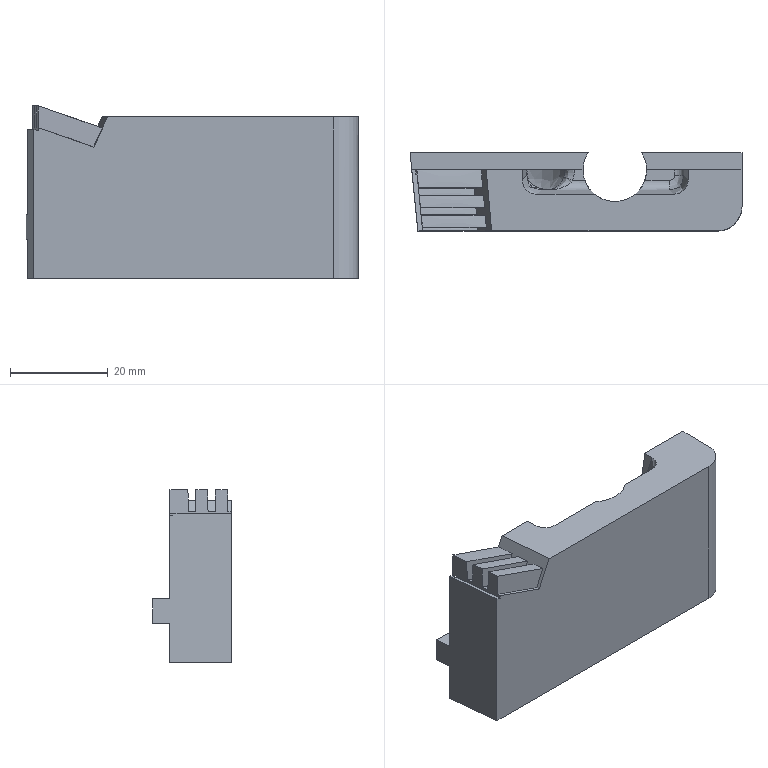Part | STEP file | P011002M005-000 | 1 solid | 59 faces | box 67.862 x 16 x 35.33 mm | volume 24834 mm3 | spline 32 | plane 20 | cylinder 5 | other 1 | cone 1 | commonest cylinder face diameters 4 x3 10 x1 13 x1